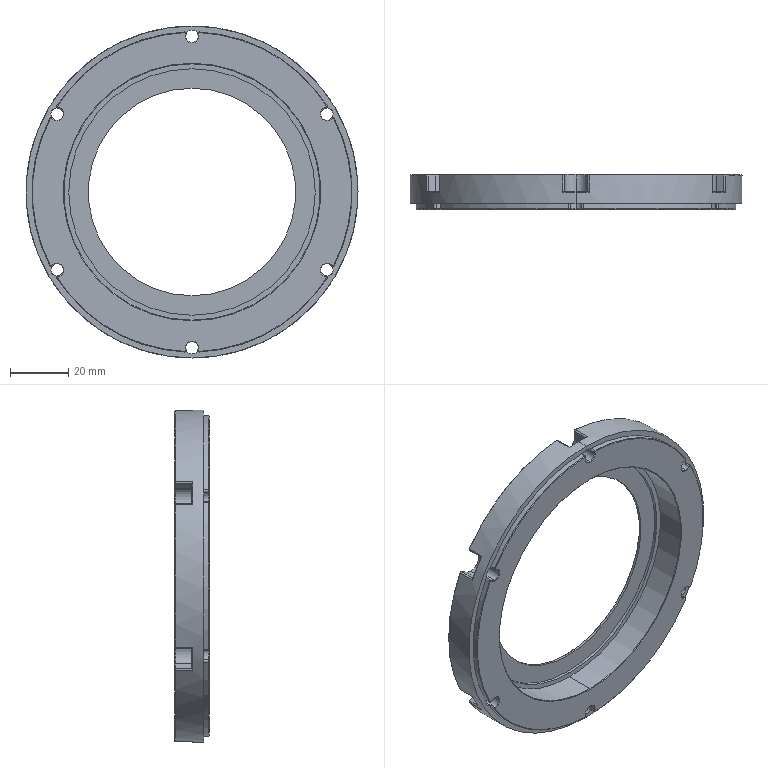Part | NX | features BREP 1 | 1 solid | 426 faces | box 114 x 12 x 114 mm | volume 46144 mm3 | cylinder 193 | cone 118 | spline 78 | plane 37 | commonest cylinder face diameters 5 x120 1 x34 4.2 x12 8 x9 110 x6 6 x4